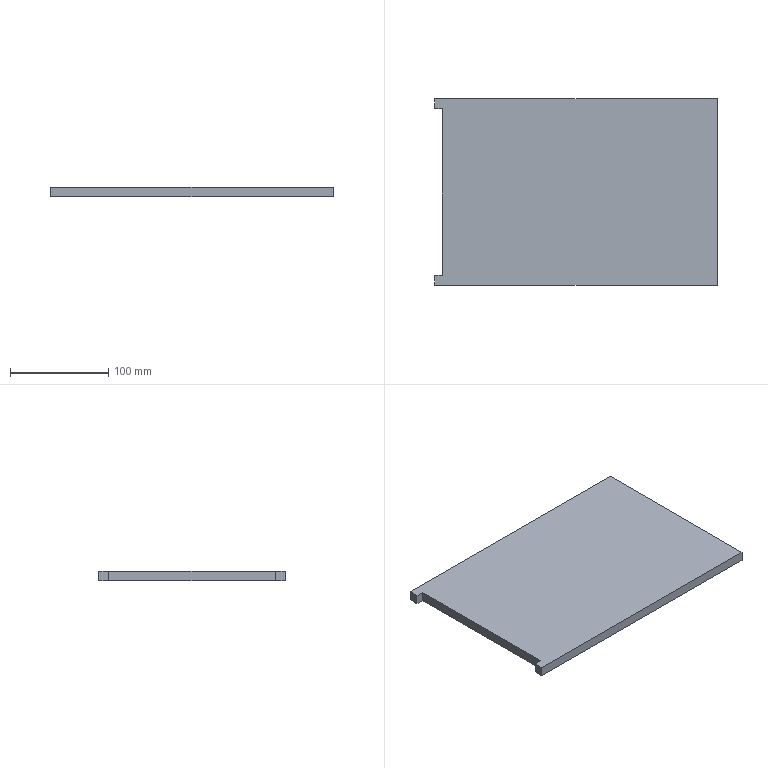Part | STEP file | 001-003-Shaft storage magazine base plate | 1 solid | 10 faces | box 288 x 190 x 10 mm | volume 533600 mm3 | plane 10
STEP:
#1=CARTESIAN_POINT('',(0.,0.,0.));
#2=DIRECTION('',(0.,0.,1.));
#3=DIRECTION('',(1.,0.,0.));
#4=AXIS2_PLACEMENT_3D('',#1,#2,#3);
#5=CARTESIAN_POINT('',(-144.,-85.,10.));
#6=VERTEX_POINT('',#5);
#7=CARTESIAN_POINT('',(-144.,-85.,0.));
#8=VERTEX_POINT('',#7);
#9=CARTESIAN_POINT('',(-144.,-85.,10.));
#10=DIRECTION('',(0.,0.,-1.));
#11=VECTOR('',#10,1.);
#12=LINE('',#9,#11);
#13=CARTESIAN_POINT('',(-144.,-95.,10.));
#14=DIRECTION('',(1.,0.,0.));
#15=DIRECTION('',(0.,0.,-1.));
#16=AXIS2_PLACEMENT_3D('',#13,#14,#15);
#17=PLANE('',#16);
#18=CARTESIAN_POINT('',(0.,10.));
#19=DIRECTION('',(1.,0.));
#20=VECTOR('',#19,1.);
#21=LINE('',#18,#20);
#22=(GEOMETRIC_REPRESENTATION_CONTEXT(2)PARAMETRIC_REPRESENTATION_CONTEXT()REPRESENTATION_CONTEXT('',''));
#23=DEFINITIONAL_REPRESENTATION('',(#21),#22);
#24=PCURVE('',#17,#23);
#25=CARTESIAN_POINT('',(-144.,-85.,10.));
#26=DIRECTION('',(0.,1.,0.));
#27=DIRECTION('',(0.,0.,1.));
#28=AXIS2_PLACEMENT_3D('',#25,#26,#27);
#29=PLANE('',#28);
#30=CARTESIAN_POINT('',(0.,0.));
#31=DIRECTION('',(-1.,0.));
#32=VECTOR('',#31,1.);
#33=LINE('',#30,#32);
#34=(GEOMETRIC_REPRESENTATION_CONTEXT(2)PARAMETRIC_REPRESENTATION_CONTEXT()REPRESENTATION_CONTEXT('',''));
#35=DEFINITIONAL_REPRESENTATION('',(#33),#34);
#36=PCURVE('',#29,#35);
#37=SURFACE_CURVE('',#12,(#24,#36),.PCURVE_S1.);
#38=EDGE_CURVE('',#6,#8,#37,.T.);
#39=ORIENTED_EDGE('',*,*,#38,.T.);
#40=CARTESIAN_POINT('',(-144.,-95.,0.));
#41=VERTEX_POINT('',#40);
#42=CARTESIAN_POINT('',(-144.,-95.,0.));
#43=DIRECTION('',(0.,-1.,0.));
#44=VECTOR('',#43,1.);
#45=LINE('',#42,#44);
#46=CARTESIAN_POINT('',(10.,0.));
#47=DIRECTION('',(0.,-1.));
#48=VECTOR('',#47,1.);
#49=LINE('',#46,#48);
#50=(GEOMETRIC_REPRESENTATION_CONTEXT(2)PARAMETRIC_REPRESENTATION_CONTEXT()REPRESENTATION_CONTEXT('',''));
#51=DEFINITIONAL_REPRESENTATION('',(#49),#50);
#52=PCURVE('',#17,#51);
#53=CARTESIAN_POINT('',(0.,0.,0.));
#54=DIRECTION('',(0.,0.,-1.));
#55=DIRECTION('',(-1.,0.,0.));
#56=AXIS2_PLACEMENT_3D('',#53,#54,#55);
#57=PLANE('',#56);
#58=CARTESIAN_POINT('',(144.,-95.));
#59=DIRECTION('',(0.,-1.));
#60=VECTOR('',#59,1.);
#61=LINE('',#58,#60);
#62=(GEOMETRIC_REPRESENTATION_CONTEXT(2)PARAMETRIC_REPRESENTATION_CONTEXT()REPRESENTATION_CONTEXT('',''));
#63=DEFINITIONAL_REPRESENTATION('',(#61),#62);
#64=PCURVE('',#57,#63);
#65=SURFACE_CURVE('',#45,(#52,#64),.PCURVE_S1.);
#66=EDGE_CURVE('',#8,#41,#65,.T.);
#67=ORIENTED_EDGE('',*,*,#66,.T.);
#68=CARTESIAN_POINT('',(-144.,-95.,10.));
#69=VERTEX_POINT('',#68);
#70=CARTESIAN_POINT('',(-144.,-95.,10.));
#71=DIRECTION('',(0.,0.,-1.));
#72=VECTOR('',#71,1.);
#73=LINE('',#70,#72);
#74=CARTESIAN_POINT('',(0.,0.));
#75=DIRECTION('',(1.,0.));
#76=VECTOR('',#75,1.);
#77=LINE('',#74,#76);
#78=(GEOMETRIC_REPRESENTATION_CONTEXT(2)PARAMETRIC_REPRESENTATION_CONTEXT()REPRESENTATION_CONTEXT('',''));
#79=DEFINITIONAL_REPRESENTATION('',(#77),#78);
#80=PCURVE('',#17,#79);
#81=CARTESIAN_POINT('',(-144.,-95.,10.));
#82=DIRECTION('',(0.,1.,0.));
#83=DIRECTION('',(0.,0.,1.));
#84=AXIS2_PLACEMENT_3D('',#81,#82,#83);
#85=PLANE('',#84);
#86=CARTESIAN_POINT('',(0.,0.));
#87=DIRECTION('',(-1.,0.));
#88=VECTOR('',#87,1.);
#89=LINE('',#86,#88);
#90=(GEOMETRIC_REPRESENTATION_CONTEXT(2)PARAMETRIC_REPRESENTATION_CONTEXT()REPRESENTATION_CONTEXT('',''));
#91=DEFINITIONAL_REPRESENTATION('',(#89),#90);
#92=PCURVE('',#85,#91);
#93=SURFACE_CURVE('',#73,(#80,#92),.PCURVE_S1.);
#94=EDGE_CURVE('',#69,#41,#93,.T.);
#95=ORIENTED_EDGE('',*,*,#94,.F.);
#96=CARTESIAN_POINT('',(-144.,-95.,10.));
#97=DIRECTION('',(0.,-1.,0.));
#98=VECTOR('',#97,1.);
#99=LINE('',#96,#98);
#100=CARTESIAN_POINT('',(0.,0.));
#101=DIRECTION('',(0.,-1.));
#102=VECTOR('',#101,1.);
#103=LINE('',#100,#102);
#104=(GEOMETRIC_REPRESENTATION_CONTEXT(2)PARAMETRIC_REPRESENTATION_CONTEXT()REPRESENTATION_CONTEXT('',''));
#105=DEFINITIONAL_REPRESENTATION('',(#103),#104);
#106=PCURVE('',#17,#105);
#107=CARTESIAN_POINT('',(0.,0.,10.));
#108=DIRECTION('',(0.,0.,-1.));
#109=DIRECTION('',(-1.,0.,0.));
#110=AXIS2_PLACEMENT_3D('',#107,#108,#109);
#111=PLANE('',#110);
#112=CARTESIAN_POINT('',(144.,-95.));
#113=DIRECTION('',(0.,-1.));
#114=VECTOR('',#113,1.);
#115=LINE('',#112,#114);
#116=(GEOMETRIC_REPRESENTATION_CONTEXT(2)PARAMETRIC_REPRESENTATION_CONTEXT()REPRESENTATION_CONTEXT('',''));
#117=DEFINITIONAL_REPRESENTATION('',(#115),#116);
#118=PCURVE('',#111,#117);
#119=SURFACE_CURVE('',#99,(#106,#118),.PCURVE_S1.);
#120=EDGE_CURVE('',#6,#69,#119,.T.);
#121=ORIENTED_EDGE('',*,*,#120,.F.);
#122=EDGE_LOOP('',(#39,#67,#95,#121));
#123=FACE_BOUND('',#122,.T.);
#124=ADVANCED_FACE('',(#123),#17,.F.);
#125=CARTESIAN_POINT('',(-144.,85.,10.));
#126=VERTEX_POINT('',#125);
#127=CARTESIAN_POINT('',(-144.,85.,0.));
#128=VERTEX_POINT('',#127);
#129=CARTESIAN_POINT('',(-144.,85.,10.));
#130=DIRECTION('',(0.,0.,-1.));
#131=VECTOR('',#130,1.);
#132=LINE('',#129,#131);
#133=CARTESIAN_POINT('',(-144.,-95.,10.));
#134=DIRECTION('',(1.,0.,0.));
#135=DIRECTION('',(0.,0.,-1.));
#136=AXIS2_PLACEMENT_3D('',#133,#134,#135);
#137=PLANE('',#136);
#138=CARTESIAN_POINT('',(0.,180.));
#139=DIRECTION('',(1.,0.));
#140=VECTOR('',#139,1.);
#141=LINE('',#138,#140);
#142=(GEOMETRIC_REPRESENTATION_CONTEXT(2)PARAMETRIC_REPRESENTATION_CONTEXT()REPRESENTATION_CONTEXT('',''));
#143=DEFINITIONAL_REPRESENTATION('',(#141),#142);
#144=PCURVE('',#137,#143);
#145=CARTESIAN_POINT('',(-144.,85.,10.));
#146=DIRECTION('',(0.,-1.,0.));
#147=DIRECTION('',(1.,0.,0.));
#148=AXIS2_PLACEMENT_3D('',#145,#146,#147);
#149=PLANE('',#148);
#150=CARTESIAN_POINT('',(0.,0.));
#151=DIRECTION('',(0.,-1.));
#152=VECTOR('',#151,1.);
#153=LINE('',#150,#152);
#154=(GEOMETRIC_REPRESENTATION_CONTEXT(2)PARAMETRIC_REPRESENTATION_CONTEXT()REPRESENTATION_CONTEXT('',''));
#155=DEFINITIONAL_REPRESENTATION('',(#153),#154);
#156=PCURVE('',#149,#155);
#157=SURFACE_CURVE('',#132,(#144,#156),.PCURVE_S1.);
#158=EDGE_CURVE('',#126,#128,#157,.T.);
#159=ORIENTED_EDGE('',*,*,#158,.F.);
#160=CARTESIAN_POINT('',(-144.,95.,10.));
#161=VERTEX_POINT('',#160);
#162=CARTESIAN_POINT('',(-144.,-95.,10.));
#163=DIRECTION('',(0.,-1.,0.));
#164=VECTOR('',#163,1.);
#165=LINE('',#162,#164);
#166=CARTESIAN_POINT('',(0.,0.));
#167=DIRECTION('',(0.,-1.));
#168=VECTOR('',#167,1.);
#169=LINE('',#166,#168);
#170=(GEOMETRIC_REPRESENTATION_CONTEXT(2)PARAMETRIC_REPRESENTATION_CONTEXT()REPRESENTATION_CONTEXT('',''));
#171=DEFINITIONAL_REPRESENTATION('',(#169),#170);
#172=PCURVE('',#137,#171);
#173=CARTESIAN_POINT('',(144.,-95.));
#174=DIRECTION('',(0.,-1.));
#175=VECTOR('',#174,1.);
#176=LINE('',#173,#175);
#177=(GEOMETRIC_REPRESENTATION_CONTEXT(2)PARAMETRIC_REPRESENTATION_CONTEXT()REPRESENTATION_CONTEXT('',''));
#178=DEFINITIONAL_REPRESENTATION('',(#176),#177);
#179=PCURVE('',#111,#178);
#180=SURFACE_CURVE('',#165,(#172,#179),.PCURVE_S1.);
#181=EDGE_CURVE('',#161,#126,#180,.T.);
#182=ORIENTED_EDGE('',*,*,#181,.F.);
#183=CARTESIAN_POINT('',(-144.,95.,0.));
#184=VERTEX_POINT('',#183);
#185=CARTESIAN_POINT('',(-144.,95.,10.));
#186=DIRECTION('',(0.,0.,-1.));
#187=VECTOR('',#186,1.);
#188=LINE('',#185,#187);
#189=CARTESIAN_POINT('',(0.,190.));
#190=DIRECTION('',(1.,0.));
#191=VECTOR('',#190,1.);
#192=LINE('',#189,#191);
#193=(GEOMETRIC_REPRESENTATION_CONTEXT(2)PARAMETRIC_REPRESENTATION_CONTEXT()REPRESENTATION_CONTEXT('',''));
#194=DEFINITIONAL_REPRESENTATION('',(#192),#193);
#195=PCURVE('',#137,#194);
#196=CARTESIAN_POINT('',(-144.,95.,10.));
#197=DIRECTION('',(0.,-1.,0.));
#198=DIRECTION('',(0.,0.,-1.));
#199=AXIS2_PLACEMENT_3D('',#196,#197,#198);
#200=PLANE('',#199);
#201=CARTESIAN_POINT('',(0.,0.));
#202=DIRECTION('',(1.,0.));
#203=VECTOR('',#202,1.);
#204=LINE('',#201,#203);
#205=(GEOMETRIC_REPRESENTATION_CONTEXT(2)PARAMETRIC_REPRESENTATION_CONTEXT()REPRESENTATION_CONTEXT('',''));
#206=DEFINITIONAL_REPRESENTATION('',(#204),#205);
#207=PCURVE('',#200,#206);
#208=SURFACE_CURVE('',#188,(#195,#207),.PCURVE_S1.);
#209=EDGE_CURVE('',#161,#184,#208,.T.);
#210=ORIENTED_EDGE('',*,*,#209,.T.);
#211=CARTESIAN_POINT('',(-144.,-95.,0.));
#212=DIRECTION('',(0.,-1.,0.));
#213=VECTOR('',#212,1.);
#214=LINE('',#211,#213);
#215=CARTESIAN_POINT('',(10.,0.));
#216=DIRECTION('',(0.,-1.));
#217=VECTOR('',#216,1.);
#218=LINE('',#215,#217);
#219=(GEOMETRIC_REPRESENTATION_CONTEXT(2)PARAMETRIC_REPRESENTATION_CONTEXT()REPRESENTATION_CONTEXT('',''));
#220=DEFINITIONAL_REPRESENTATION('',(#218),#219);
#221=PCURVE('',#137,#220);
#222=CARTESIAN_POINT('',(144.,-95.));
#223=DIRECTION('',(0.,-1.));
#224=VECTOR('',#223,1.);
#225=LINE('',#222,#224);
#226=(GEOMETRIC_REPRESENTATION_CONTEXT(2)PARAMETRIC_REPRESENTATION_CONTEXT()REPRESENTATION_CONTEXT('',''));
#227=DEFINITIONAL_REPRESENTATION('',(#225),#226);
#228=PCURVE('',#57,#227);
#229=SURFACE_CURVE('',#214,(#221,#228),.PCURVE_S1.);
#230=EDGE_CURVE('',#184,#128,#229,.T.);
#231=ORIENTED_EDGE('',*,*,#230,.T.);
#232=EDGE_LOOP('',(#159,#182,#210,#231));
#233=FACE_BOUND('',#232,.T.);
#234=ADVANCED_FACE('',(#233),#137,.F.);
#235=CARTESIAN_POINT('',(-136.,-85.,10.));
#236=VERTEX_POINT('',#235);
#237=CARTESIAN_POINT('',(-144.,-85.,10.));
#238=DIRECTION('',(1.,0.,0.));
#239=VECTOR('',#238,1.);
#240=LINE('',#237,#239);
#241=CARTESIAN_POINT('',(144.,-85.));
#242=DIRECTION('',(-1.,0.));
#243=VECTOR('',#242,1.);
#244=LINE('',#241,#243);
#245=(GEOMETRIC_REPRESENTATION_CONTEXT(2)PARAMETRIC_REPRESENTATION_CONTEXT()REPRESENTATION_CONTEXT('',''));
#246=DEFINITIONAL_REPRESENTATION('',(#244),#245);
#247=PCURVE('',#111,#246);
#248=CARTESIAN_POINT('',(0.,0.));
#249=DIRECTION('',(0.,1.));
#250=VECTOR('',#249,1.);
#251=LINE('',#248,#250);
#252=(GEOMETRIC_REPRESENTATION_CONTEXT(2)PARAMETRIC_REPRESENTATION_CONTEXT()REPRESENTATION_CONTEXT('',''));
#253=DEFINITIONAL_REPRESENTATION('',(#251),#252);
#254=PCURVE('',#29,#253);
#255=SURFACE_CURVE('',#240,(#247,#254),.PCURVE_S1.);
#256=EDGE_CURVE('',#6,#236,#255,.T.);
#257=ORIENTED_EDGE('',*,*,#256,.F.);
#258=ORIENTED_EDGE('',*,*,#120,.T.);
#259=CARTESIAN_POINT('',(144.,-95.,10.));
#260=VERTEX_POINT('',#259);
#261=CARTESIAN_POINT('',(-144.,-95.,10.));
#262=DIRECTION('',(1.,0.,0.));
#263=VECTOR('',#262,1.);
#264=LINE('',#261,#263);
#265=CARTESIAN_POINT('',(144.,-95.));
#266=DIRECTION('',(-1.,0.));
#267=VECTOR('',#266,1.);
#268=LINE('',#265,#267);
#269=(GEOMETRIC_REPRESENTATION_CONTEXT(2)PARAMETRIC_REPRESENTATION_CONTEXT()REPRESENTATION_CONTEXT('',''));
#270=DEFINITIONAL_REPRESENTATION('',(#268),#269);
#271=PCURVE('',#111,#270);
#272=CARTESIAN_POINT('',(0.,0.));
#273=DIRECTION('',(0.,1.));
#274=VECTOR('',#273,1.);
#275=LINE('',#272,#274);
#276=(GEOMETRIC_REPRESENTATION_CONTEXT(2)PARAMETRIC_REPRESENTATION_CONTEXT()REPRESENTATION_CONTEXT('',''));
#277=DEFINITIONAL_REPRESENTATION('',(#275),#276);
#278=PCURVE('',#85,#277);
#279=SURFACE_CURVE('',#264,(#271,#278),.PCURVE_S1.);
#280=EDGE_CURVE('',#69,#260,#279,.T.);
#281=ORIENTED_EDGE('',*,*,#280,.T.);
#282=CARTESIAN_POINT('',(144.,95.,10.));
#283=VERTEX_POINT('',#282);
#284=CARTESIAN_POINT('',(144.,-95.,10.));
#285=DIRECTION('',(0.,1.,0.));
#286=VECTOR('',#285,1.);
#287=LINE('',#284,#286);
#288=CARTESIAN_POINT('',(-144.,-95.));
#289=DIRECTION('',(0.,1.));
#290=VECTOR('',#289,1.);
#291=LINE('',#288,#290);
#292=(GEOMETRIC_REPRESENTATION_CONTEXT(2)PARAMETRIC_REPRESENTATION_CONTEXT()REPRESENTATION_CONTEXT('',''));
#293=DEFINITIONAL_REPRESENTATION('',(#291),#292);
#294=PCURVE('',#111,#293);
#295=CARTESIAN_POINT('',(144.,-95.,10.));
#296=DIRECTION('',(-1.,0.,0.));
#297=DIRECTION('',(0.,0.,1.));
#298=AXIS2_PLACEMENT_3D('',#295,#296,#297);
#299=PLANE('',#298);
#300=CARTESIAN_POINT('',(0.,0.));
#301=DIRECTION('',(0.,1.));
#302=VECTOR('',#301,1.);
#303=LINE('',#300,#302);
#304=(GEOMETRIC_REPRESENTATION_CONTEXT(2)PARAMETRIC_REPRESENTATION_CONTEXT()REPRESENTATION_CONTEXT('',''));
#305=DEFINITIONAL_REPRESENTATION('',(#303),#304);
#306=PCURVE('',#299,#305);
#307=SURFACE_CURVE('',#287,(#294,#306),.PCURVE_S1.);
#308=EDGE_CURVE('',#260,#283,#307,.T.);
#309=ORIENTED_EDGE('',*,*,#308,.T.);
#310=CARTESIAN_POINT('',(-144.,95.,10.));
#311=DIRECTION('',(-1.,0.,0.));
#312=VECTOR('',#311,1.);
#313=LINE('',#310,#312);
#314=CARTESIAN_POINT('',(144.,95.));
#315=DIRECTION('',(1.,0.));
#316=VECTOR('',#315,1.);
#317=LINE('',#314,#316);
#318=(GEOMETRIC_REPRESENTATION_CONTEXT(2)PARAMETRIC_REPRESENTATION_CONTEXT()REPRESENTATION_CONTEXT('',''));
#319=DEFINITIONAL_REPRESENTATION('',(#317),#318);
#320=PCURVE('',#111,#319);
#321=CARTESIAN_POINT('',(0.,0.));
#322=DIRECTION('',(0.,-1.));
#323=VECTOR('',#322,1.);
#324=LINE('',#321,#323);
#325=(GEOMETRIC_REPRESENTATION_CONTEXT(2)PARAMETRIC_REPRESENTATION_CONTEXT()REPRESENTATION_CONTEXT('',''));
#326=DEFINITIONAL_REPRESENTATION('',(#324),#325);
#327=PCURVE('',#200,#326);
#328=SURFACE_CURVE('',#313,(#320,#327),.PCURVE_S1.);
#329=EDGE_CURVE('',#283,#161,#328,.T.);
#330=ORIENTED_EDGE('',*,*,#329,.T.);
#331=ORIENTED_EDGE('',*,*,#181,.T.);
#332=CARTESIAN_POINT('',(-136.,85.,10.));
#333=VERTEX_POINT('',#332);
#334=CARTESIAN_POINT('',(-144.,85.,10.));
#335=DIRECTION('',(-1.,0.,0.));
#336=VECTOR('',#335,1.);
#337=LINE('',#334,#336);
#338=CARTESIAN_POINT('',(144.,85.));
#339=DIRECTION('',(1.,0.));
#340=VECTOR('',#339,1.);
#341=LINE('',#338,#340);
#342=(GEOMETRIC_REPRESENTATION_CONTEXT(2)PARAMETRIC_REPRESENTATION_CONTEXT()REPRESENTATION_CONTEXT('',''));
#343=DEFINITIONAL_REPRESENTATION('',(#341),#342);
#344=PCURVE('',#111,#343);
#345=CARTESIAN_POINT('',(0.,0.));
#346=DIRECTION('',(-1.,0.));
#347=VECTOR('',#346,1.);
#348=LINE('',#345,#347);
#349=(GEOMETRIC_REPRESENTATION_CONTEXT(2)PARAMETRIC_REPRESENTATION_CONTEXT()REPRESENTATION_CONTEXT('',''));
#350=DEFINITIONAL_REPRESENTATION('',(#348),#349);
#351=PCURVE('',#149,#350);
#352=SURFACE_CURVE('',#337,(#344,#351),.PCURVE_S1.);
#353=EDGE_CURVE('',#333,#126,#352,.T.);
#354=ORIENTED_EDGE('',*,*,#353,.F.);
#355=CARTESIAN_POINT('',(-136.,85.,10.));
#356=DIRECTION('',(0.,1.,0.));
#357=VECTOR('',#356,1.);
#358=LINE('',#355,#357);
#359=CARTESIAN_POINT('',(136.,85.));
#360=DIRECTION('',(0.,1.));
#361=VECTOR('',#360,1.);
#362=LINE('',#359,#361);
#363=(GEOMETRIC_REPRESENTATION_CONTEXT(2)PARAMETRIC_REPRESENTATION_CONTEXT()REPRESENTATION_CONTEXT('',''));
#364=DEFINITIONAL_REPRESENTATION('',(#362),#363);
#365=PCURVE('',#111,#364);
#366=CARTESIAN_POINT('',(-136.,85.,10.));
#367=DIRECTION('',(-1.,0.,0.));
#368=DIRECTION('',(0.,0.,1.));
#369=AXIS2_PLACEMENT_3D('',#366,#367,#368);
#370=PLANE('',#369);
#371=CARTESIAN_POINT('',(0.,0.));
#372=DIRECTION('',(0.,1.));
#373=VECTOR('',#372,1.);
#374=LINE('',#371,#373);
#375=(GEOMETRIC_REPRESENTATION_CONTEXT(2)PARAMETRIC_REPRESENTATION_CONTEXT()REPRESENTATION_CONTEXT('',''));
#376=DEFINITIONAL_REPRESENTATION('',(#374),#375);
#377=PCURVE('',#370,#376);
#378=SURFACE_CURVE('',#358,(#365,#377),.PCURVE_S1.);
#379=EDGE_CURVE('',#236,#333,#378,.T.);
#380=ORIENTED_EDGE('',*,*,#379,.F.);
#381=EDGE_LOOP('',(#257,#258,#281,#309,#330,#331,#354,#380));
#382=FACE_BOUND('',#381,.T.);
#383=ADVANCED_FACE('',(#382),#111,.F.);
#384=ORIENTED_EDGE('',*,*,#66,.F.);
#385=CARTESIAN_POINT('',(-136.,-85.,0.));
#386=VERTEX_POINT('',#385);
#387=CARTESIAN_POINT('',(-144.,-85.,0.));
#388=DIRECTION('',(1.,0.,0.));
#389=VECTOR('',#388,1.);
#390=LINE('',#387,#389);
#391=CARTESIAN_POINT('',(144.,-85.));
#392=DIRECTION('',(-1.,0.));
#393=VECTOR('',#392,1.);
#394=LINE('',#391,#393);
#395=(GEOMETRIC_REPRESENTATION_CONTEXT(2)PARAMETRIC_REPRESENTATION_CONTEXT()REPRESENTATION_CONTEXT('',''));
#396=DEFINITIONAL_REPRESENTATION('',(#394),#395);
#397=PCURVE('',#57,#396);
#398=CARTESIAN_POINT('',(-10.,0.));
#399=DIRECTION('',(0.,1.));
#400=VECTOR('',#399,1.);
#401=LINE('',#398,#400);
#402=(GEOMETRIC_REPRESENTATION_CONTEXT(2)PARAMETRIC_REPRESENTATION_CONTEXT()REPRESENTATION_CONTEXT('',''));
#403=DEFINITIONAL_REPRESENTATION('',(#401),#402);
#404=PCURVE('',#29,#403);
#405=SURFACE_CURVE('',#390,(#397,#404),.PCURVE_S1.);
#406=EDGE_CURVE('',#8,#386,#405,.T.);
#407=ORIENTED_EDGE('',*,*,#406,.T.);
#408=CARTESIAN_POINT('',(-136.,85.,0.));
#409=VERTEX_POINT('',#408);
#410=CARTESIAN_POINT('',(-136.,85.,0.));
#411=DIRECTION('',(0.,1.,0.));
#412=VECTOR('',#411,1.);
#413=LINE('',#410,#412);
#414=CARTESIAN_POINT('',(136.,85.));
#415=DIRECTION('',(0.,1.));
#416=VECTOR('',#415,1.);
#417=LINE('',#414,#416);
#418=(GEOMETRIC_REPRESENTATION_CONTEXT(2)PARAMETRIC_REPRESENTATION_CONTEXT()REPRESENTATION_CONTEXT('',''));
#419=DEFINITIONAL_REPRESENTATION('',(#417),#418);
#420=PCURVE('',#57,#419);
#421=CARTESIAN_POINT('',(-10.,0.));
#422=DIRECTION('',(0.,1.));
#423=VECTOR('',#422,1.);
#424=LINE('',#421,#423);
#425=(GEOMETRIC_REPRESENTATION_CONTEXT(2)PARAMETRIC_REPRESENTATION_CONTEXT()REPRESENTATION_CONTEXT('',''));
#426=DEFINITIONAL_REPRESENTATION('',(#424),#425);
#427=PCURVE('',#370,#426);
#428=SURFACE_CURVE('',#413,(#420,#427),.PCURVE_S1.);
#429=EDGE_CURVE('',#386,#409,#428,.T.);
#430=ORIENTED_EDGE('',*,*,#429,.T.);
#431=CARTESIAN_POINT('',(-144.,85.,0.));
#432=DIRECTION('',(-1.,0.,0.));
#433=VECTOR('',#432,1.);
#434=LINE('',#431,#433);
#435=CARTESIAN_POINT('',(144.,85.));
#436=DIRECTION('',(1.,0.));
#437=VECTOR('',#436,1.);
#438=LINE('',#435,#437);
#439=(GEOMETRIC_REPRESENTATION_CONTEXT(2)PARAMETRIC_REPRESENTATION_CONTEXT()REPRESENTATION_CONTEXT('',''));
#440=DEFINITIONAL_REPRESENTATION('',(#438),#439);
#441=PCURVE('',#57,#440);
#442=CARTESIAN_POINT('',(0.,-10.));
#443=DIRECTION('',(-1.,0.));
#444=VECTOR('',#443,1.);
#445=LINE('',#442,#444);
#446=(GEOMETRIC_REPRESENTATION_CONTEXT(2)PARAMETRIC_REPRESENTATION_CONTEXT()REPRESENTATION_CONTEXT('',''));
#447=DEFINITIONAL_REPRESENTATION('',(#445),#446);
#448=PCURVE('',#149,#447);
#449=SURFACE_CURVE('',#434,(#441,#448),.PCURVE_S1.);
#450=EDGE_CURVE('',#409,#128,#449,.T.);
#451=ORIENTED_EDGE('',*,*,#450,.T.);
#452=ORIENTED_EDGE('',*,*,#230,.F.);
#453=CARTESIAN_POINT('',(144.,95.,0.));
#454=VERTEX_POINT('',#453);
#455=CARTESIAN_POINT('',(-144.,95.,0.));
#456=DIRECTION('',(-1.,0.,0.));
#457=VECTOR('',#456,1.);
#458=LINE('',#455,#457);
#459=CARTESIAN_POINT('',(144.,95.));
#460=DIRECTION('',(1.,0.));
#461=VECTOR('',#460,1.);
#462=LINE('',#459,#461);
#463=(GEOMETRIC_REPRESENTATION_CONTEXT(2)PARAMETRIC_REPRESENTATION_CONTEXT()REPRESENTATION_CONTEXT('',''));
#464=DEFINITIONAL_REPRESENTATION('',(#462),#463);
#465=PCURVE('',#57,#464);
#466=CARTESIAN_POINT('',(10.,0.));
#467=DIRECTION('',(0.,-1.));
#468=VECTOR('',#467,1.);
#469=LINE('',#466,#468);
#470=(GEOMETRIC_REPRESENTATION_CONTEXT(2)PARAMETRIC_REPRESENTATION_CONTEXT()REPRESENTATION_CONTEXT('',''));
#471=DEFINITIONAL_REPRESENTATION('',(#469),#470);
#472=PCURVE('',#200,#471);
#473=SURFACE_CURVE('',#458,(#465,#472),.PCURVE_S1.);
#474=EDGE_CURVE('',#454,#184,#473,.T.);
#475=ORIENTED_EDGE('',*,*,#474,.F.);
#476=CARTESIAN_POINT('',(144.,-95.,0.));
#477=VERTEX_POINT('',#476);
#478=CARTESIAN_POINT('',(144.,-95.,0.));
#479=DIRECTION('',(0.,1.,0.));
#480=VECTOR('',#479,1.);
#481=LINE('',#478,#480);
#482=CARTESIAN_POINT('',(-144.,-95.));
#483=DIRECTION('',(0.,1.));
#484=VECTOR('',#483,1.);
#485=LINE('',#482,#484);
#486=(GEOMETRIC_REPRESENTATION_CONTEXT(2)PARAMETRIC_REPRESENTATION_CONTEXT()REPRESENTATION_CONTEXT('',''));
#487=DEFINITIONAL_REPRESENTATION('',(#485),#486);
#488=PCURVE('',#57,#487);
#489=CARTESIAN_POINT('',(-10.,0.));
#490=DIRECTION('',(0.,1.));
#491=VECTOR('',#490,1.);
#492=LINE('',#489,#491);
#493=(GEOMETRIC_REPRESENTATION_CONTEXT(2)PARAMETRIC_REPRESENTATION_CONTEXT()REPRESENTATION_CONTEXT('',''));
#494=DEFINITIONAL_REPRESENTATION('',(#492),#493);
#495=PCURVE('',#299,#494);
#496=SURFACE_CURVE('',#481,(#488,#495),.PCURVE_S1.);
#497=EDGE_CURVE('',#477,#454,#496,.T.);
#498=ORIENTED_EDGE('',*,*,#497,.F.);
#499=CARTESIAN_POINT('',(-144.,-95.,0.));
#500=DIRECTION('',(1.,0.,0.));
#501=VECTOR('',#500,1.);
#502=LINE('',#499,#501);
#503=CARTESIAN_POINT('',(144.,-95.));
#504=DIRECTION('',(-1.,0.));
#505=VECTOR('',#504,1.);
#506=LINE('',#503,#505);
#507=(GEOMETRIC_REPRESENTATION_CONTEXT(2)PARAMETRIC_REPRESENTATION_CONTEXT()REPRESENTATION_CONTEXT('',''));
#508=DEFINITIONAL_REPRESENTATION('',(#506),#507);
#509=PCURVE('',#57,#508);
#510=CARTESIAN_POINT('',(-10.,0.));
#511=DIRECTION('',(0.,1.));
#512=VECTOR('',#511,1.);
#513=LINE('',#510,#512);
#514=(GEOMETRIC_REPRESENTATION_CONTEXT(2)PARAMETRIC_REPRESENTATION_CONTEXT()REPRESENTATION_CONTEXT('',''));
#515=DEFINITIONAL_REPRESENTATION('',(#513),#514);
#516=PCURVE('',#85,#515);
#517=SURFACE_CURVE('',#502,(#509,#516),.PCURVE_S1.);
#518=EDGE_CURVE('',#41,#477,#517,.T.);
#519=ORIENTED_EDGE('',*,*,#518,.F.);
#520=EDGE_LOOP('',(#384,#407,#430,#451,#452,#475,#498,#519));
#521=FACE_BOUND('',#520,.T.);
#522=ADVANCED_FACE('',(#521),#57,.T.);
#523=ORIENTED_EDGE('',*,*,#497,.T.);
#524=CARTESIAN_POINT('',(144.,95.,10.));
#525=DIRECTION('',(0.,0.,-1.));
#526=VECTOR('',#525,1.);
#527=LINE('',#524,#526);
#528=CARTESIAN_POINT('',(0.,190.));
#529=DIRECTION('',(-1.,0.));
#530=VECTOR('',#529,1.);
#531=LINE('',#528,#530);
#532=(GEOMETRIC_REPRESENTATION_CONTEXT(2)PARAMETRIC_REPRESENTATION_CONTEXT()REPRESENTATION_CONTEXT('',''));
#533=DEFINITIONAL_REPRESENTATION('',(#531),#532);
#534=PCURVE('',#299,#533);
#535=CARTESIAN_POINT('',(0.,288.));
#536=DIRECTION('',(1.,0.));
#537=VECTOR('',#536,1.);
#538=LINE('',#535,#537);
#539=(GEOMETRIC_REPRESENTATION_CONTEXT(2)PARAMETRIC_REPRESENTATION_CONTEXT()REPRESENTATION_CONTEXT('',''));
#540=DEFINITIONAL_REPRESENTATION('',(#538),#539);
#541=PCURVE('',#200,#540);
#542=SURFACE_CURVE('',#527,(#534,#541),.PCURVE_S1.);
#543=EDGE_CURVE('',#283,#454,#542,.T.);
#544=ORIENTED_EDGE('',*,*,#543,.F.);
#545=ORIENTED_EDGE('',*,*,#308,.F.);
#546=CARTESIAN_POINT('',(144.,-95.,10.));
#547=DIRECTION('',(0.,0.,-1.));
#548=VECTOR('',#547,1.);
#549=LINE('',#546,#548);
#550=CARTESIAN_POINT('',(0.,0.));
#551=DIRECTION('',(-1.,0.));
#552=VECTOR('',#551,1.);
#553=LINE('',#550,#552);
#554=(GEOMETRIC_REPRESENTATION_CONTEXT(2)PARAMETRIC_REPRESENTATION_CONTEXT()REPRESENTATION_CONTEXT('',''));
#555=DEFINITIONAL_REPRESENTATION('',(#553),#554);
#556=PCURVE('',#299,#555);
#557=CARTESIAN_POINT('',(0.,288.));
#558=DIRECTION('',(-1.,0.));
#559=VECTOR('',#558,1.);
#560=LINE('',#557,#559);
#561=(GEOMETRIC_REPRESENTATION_CONTEXT(2)PARAMETRIC_REPRESENTATION_CONTEXT()REPRESENTATION_CONTEXT('',''));
#562=DEFINITIONAL_REPRESENTATION('',(#560),#561);
#563=PCURVE('',#85,#562);
#564=SURFACE_CURVE('',#549,(#556,#563),.PCURVE_S1.);
#565=EDGE_CURVE('',#260,#477,#564,.T.);
#566=ORIENTED_EDGE('',*,*,#565,.T.);
#567=EDGE_LOOP('',(#523,#544,#545,#566));
#568=FACE_BOUND('',#567,.T.);
#569=ADVANCED_FACE('',(#568),#299,.F.);
#570=ORIENTED_EDGE('',*,*,#474,.T.);
#571=ORIENTED_EDGE('',*,*,#209,.F.);
#572=ORIENTED_EDGE('',*,*,#329,.F.);
#573=ORIENTED_EDGE('',*,*,#543,.T.);
#574=EDGE_LOOP('',(#570,#571,#572,#573));
#575=FACE_BOUND('',#574,.T.);
#576=ADVANCED_FACE('',(#575),#200,.F.);
#577=ORIENTED_EDGE('',*,*,#518,.T.);
#578=ORIENTED_EDGE('',*,*,#565,.F.);
#579=ORIENTED_EDGE('',*,*,#280,.F.);
#580=ORIENTED_EDGE('',*,*,#94,.T.);
#581=EDGE_LOOP('',(#577,#578,#579,#580));
#582=FACE_BOUND('',#581,.T.);
#583=ADVANCED_FACE('',(#582),#85,.F.);
#584=ORIENTED_EDGE('',*,*,#406,.F.);
#585=ORIENTED_EDGE('',*,*,#38,.F.);
#586=ORIENTED_EDGE('',*,*,#256,.T.);
#587=CARTESIAN_POINT('',(-136.,-85.,10.));
#588=DIRECTION('',(0.,0.,-1.));
#589=VECTOR('',#588,1.);
#590=LINE('',#587,#589);
#591=CARTESIAN_POINT('',(0.,8.));
#592=DIRECTION('',(-1.,0.));
#593=VECTOR('',#592,1.);
#594=LINE('',#591,#593);
#595=(GEOMETRIC_REPRESENTATION_CONTEXT(2)PARAMETRIC_REPRESENTATION_CONTEXT()REPRESENTATION_CONTEXT('',''));
#596=DEFINITIONAL_REPRESENTATION('',(#594),#595);
#597=PCURVE('',#29,#596);
#598=CARTESIAN_POINT('',(0.,-170.));
#599=DIRECTION('',(-1.,0.));
#600=VECTOR('',#599,1.);
#601=LINE('',#598,#600);
#602=(GEOMETRIC_REPRESENTATION_CONTEXT(2)PARAMETRIC_REPRESENTATION_CONTEXT()REPRESENTATION_CONTEXT('',''));
#603=DEFINITIONAL_REPRESENTATION('',(#601),#602);
#604=PCURVE('',#370,#603);
#605=SURFACE_CURVE('',#590,(#597,#604),.PCURVE_S1.);
#606=EDGE_CURVE('',#236,#386,#605,.T.);
#607=ORIENTED_EDGE('',*,*,#606,.T.);
#608=EDGE_LOOP('',(#584,#585,#586,#607));
#609=FACE_BOUND('',#608,.T.);
#610=ADVANCED_FACE('',(#609),#29,.T.);
#611=ORIENTED_EDGE('',*,*,#429,.F.);
#612=ORIENTED_EDGE('',*,*,#606,.F.);
#613=ORIENTED_EDGE('',*,*,#379,.T.);
#614=CARTESIAN_POINT('',(-136.,85.,10.));
#615=DIRECTION('',(0.,0.,-1.));
#616=VECTOR('',#615,1.);
#617=LINE('',#614,#616);
#618=CARTESIAN_POINT('',(0.,0.));
#619=DIRECTION('',(-1.,0.));
#620=VECTOR('',#619,1.);
#621=LINE('',#618,#620);
#622=(GEOMETRIC_REPRESENTATION_CONTEXT(2)PARAMETRIC_REPRESENTATION_CONTEXT()REPRESENTATION_CONTEXT('',''));
#623=DEFINITIONAL_REPRESENTATION('',(#621),#622);
#624=PCURVE('',#370,#623);
#625=CARTESIAN_POINT('',(8.,0.));
#626=DIRECTION('',(0.,-1.));
#627=VECTOR('',#626,1.);
#628=LINE('',#625,#627);
#629=(GEOMETRIC_REPRESENTATION_CONTEXT(2)PARAMETRIC_REPRESENTATION_CONTEXT()REPRESENTATION_CONTEXT('',''));
#630=DEFINITIONAL_REPRESENTATION('',(#628),#629);
#631=PCURVE('',#149,#630);
#632=SURFACE_CURVE('',#617,(#624,#631),.PCURVE_S1.);
#633=EDGE_CURVE('',#333,#409,#632,.T.);
#634=ORIENTED_EDGE('',*,*,#633,.T.);
#635=EDGE_LOOP('',(#611,#612,#613,#634));
#636=FACE_BOUND('',#635,.T.);
#637=ADVANCED_FACE('',(#636),#370,.T.);
#638=ORIENTED_EDGE('',*,*,#450,.F.);
#639=ORIENTED_EDGE('',*,*,#633,.F.);
#640=ORIENTED_EDGE('',*,*,#353,.T.);
#641=ORIENTED_EDGE('',*,*,#158,.T.);
#642=EDGE_LOOP('',(#638,#639,#640,#641));
#643=FACE_BOUND('',#642,.T.);
#644=ADVANCED_FACE('',(#643),#149,.T.);
#645=CLOSED_SHELL('',(#124,#234,#383,#522,#569,#576,#583,#610,#637,#644));
#646=MANIFOLD_SOLID_BREP('',#645);
#647=(LENGTH_UNIT()NAMED_UNIT(*)SI_UNIT(.MILLI.,.METRE.));
#648=UNCERTAINTY_MEASURE_WITH_UNIT(LENGTH_MEASURE(0.0000001),#647,'','');
#649=(NAMED_UNIT(*)PLANE_ANGLE_UNIT()SI_UNIT($,.RADIAN.));
#650=(NAMED_UNIT(*)SI_UNIT($,.STERADIAN.)SOLID_ANGLE_UNIT());
#651=(GEOMETRIC_REPRESENTATION_CONTEXT(3)GLOBAL_UNCERTAINTY_ASSIGNED_CONTEXT((#648))GLOBAL_UNIT_ASSIGNED_CONTEXT((#647,#649,#650))REPRESENTATION_CONTEXT('',''));
#652=ADVANCED_BREP_SHAPE_REPRESENTATION('',(#4,#646),#651);